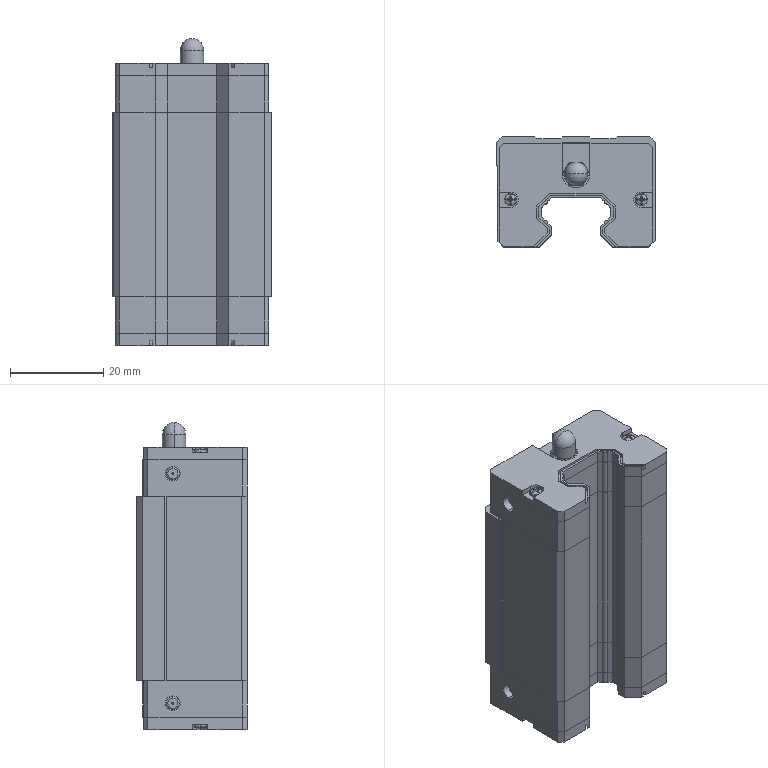Part | STEP file | 6 solids | 613 faces | box 34 x 23.6 x 65.8 mm | volume 37815 mm3 | plane 395 | spline 93 | cylinder 84 | torus 16 | cone 15 | sphere 10 | commonest cylinder face diameters 1.459 x30 3.15 x12 0.425 x8 2.638 x8 3.2 x8 4 x8